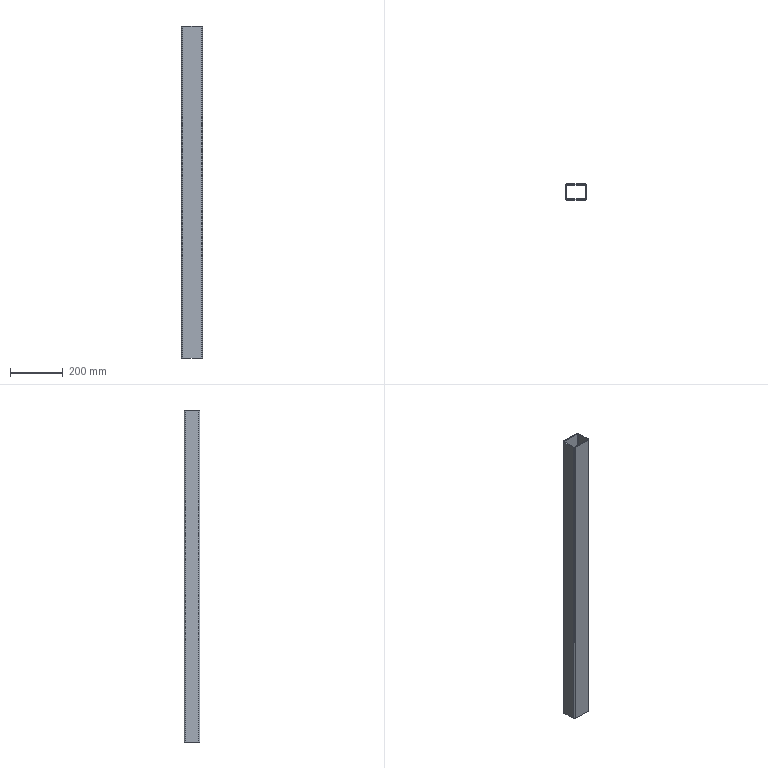Part | SolidWorks | features Extrusion 1, Fillet 1, Shell 1 | 1 solid | 18 faces | box 80 x 60 x 1264 mm | volume 993470 mm3 | plane 10 | cylinder 8 | commonest cylinder face diameters 4 x4 10 x4
STEP:
#1=CARTESIAN_POINT('',(40.,-25.,0.));
#2=VERTEX_POINT('',#1);
#3=CARTESIAN_POINT('',(40.,25.,0.));
#4=VERTEX_POINT('',#3);
#5=CARTESIAN_POINT('',(40.,30.,0.));
#6=DIRECTION('',(0.,1.,0.));
#7=VECTOR('',#6,1000.);
#8=LINE('',#5,#7);
#9=EDGE_CURVE('',#2,#4,#8,.T.);
#10=ORIENTED_EDGE('',*,*,#9,.F.);
#11=CARTESIAN_POINT('',(35.,-30.,0.));
#12=VERTEX_POINT('',#11);
#13=CARTESIAN_POINT('',(35.,-25.,0.));
#14=DIRECTION('',(0.,0.,-1.));
#15=DIRECTION('',(-1.,0.,0.));
#16=AXIS2_PLACEMENT_3D('',#13,#14,#15);
#17=CIRCLE('',#16,5.);
#18=EDGE_CURVE('',#2,#12,#17,.T.);
#19=ORIENTED_EDGE('',*,*,#18,.T.);
#20=CARTESIAN_POINT('',(-35.,-30.,0.));
#21=VERTEX_POINT('',#20);
#22=CARTESIAN_POINT('',(40.,-30.,0.));
#23=DIRECTION('',(1.,0.,0.));
#24=VECTOR('',#23,1000.);
#25=LINE('',#22,#24);
#26=EDGE_CURVE('',#21,#12,#25,.T.);
#27=ORIENTED_EDGE('',*,*,#26,.F.);
#28=CARTESIAN_POINT('',(-40.,-25.,0.));
#29=VERTEX_POINT('',#28);
#30=CARTESIAN_POINT('',(-35.,-25.,0.));
#31=DIRECTION('',(0.,0.,-1.));
#32=DIRECTION('',(-1.,0.,0.));
#33=AXIS2_PLACEMENT_3D('',#30,#31,#32);
#34=CIRCLE('',#33,5.);
#35=EDGE_CURVE('',#21,#29,#34,.T.);
#36=ORIENTED_EDGE('',*,*,#35,.T.);
#37=CARTESIAN_POINT('',(-40.,25.,0.));
#38=VERTEX_POINT('',#37);
#39=CARTESIAN_POINT('',(-40.,30.,0.));
#40=DIRECTION('',(0.,-1.,0.));
#41=VECTOR('',#40,1000.);
#42=LINE('',#39,#41);
#43=EDGE_CURVE('',#38,#29,#42,.T.);
#44=ORIENTED_EDGE('',*,*,#43,.F.);
#45=CARTESIAN_POINT('',(-35.,30.,0.));
#46=VERTEX_POINT('',#45);
#47=CARTESIAN_POINT('',(-35.,25.,0.));
#48=DIRECTION('',(0.,0.,-1.));
#49=DIRECTION('',(-1.,0.,0.));
#50=AXIS2_PLACEMENT_3D('',#47,#48,#49);
#51=CIRCLE('',#50,5.);
#52=EDGE_CURVE('',#38,#46,#51,.T.);
#53=ORIENTED_EDGE('',*,*,#52,.T.);
#54=CARTESIAN_POINT('',(35.,30.,0.));
#55=VERTEX_POINT('',#54);
#56=CARTESIAN_POINT('',(40.,30.,0.));
#57=DIRECTION('',(-1.,0.,0.));
#58=VECTOR('',#57,1000.);
#59=LINE('',#56,#58);
#60=EDGE_CURVE('',#55,#46,#59,.T.);
#61=ORIENTED_EDGE('',*,*,#60,.F.);
#62=CARTESIAN_POINT('',(35.,25.,0.));
#63=DIRECTION('',(0.,0.,-1.));
#64=DIRECTION('',(-1.,0.,0.));
#65=AXIS2_PLACEMENT_3D('',#62,#63,#64);
#66=CIRCLE('',#65,5.);
#67=EDGE_CURVE('',#55,#4,#66,.T.);
#68=ORIENTED_EDGE('',*,*,#67,.T.);
#69=EDGE_LOOP('',(#10,#19,#27,#36,#44,#53,#61,#68));
#70=FACE_OUTER_BOUND('',#69,.T.);
#71=CARTESIAN_POINT('',(37.,-25.,0.));
#72=VERTEX_POINT('',#71);
#73=CARTESIAN_POINT('',(35.,-27.,0.));
#74=VERTEX_POINT('',#73);
#75=CARTESIAN_POINT('',(35.,-25.,0.));
#76=DIRECTION('',(0.,0.,-1.));
#77=DIRECTION('',(-1.,0.,0.));
#78=AXIS2_PLACEMENT_3D('',#75,#76,#77);
#79=CIRCLE('',#78,2.);
#80=EDGE_CURVE('',#72,#74,#79,.T.);
#81=ORIENTED_EDGE('',*,*,#80,.F.);
#82=CARTESIAN_POINT('',(37.,25.,0.));
#83=VERTEX_POINT('',#82);
#84=CARTESIAN_POINT('',(37.,0.,0.));
#85=DIRECTION('',(0.,1.,0.));
#86=VECTOR('',#85,1000.);
#87=LINE('',#84,#86);
#88=EDGE_CURVE('',#72,#83,#87,.T.);
#89=ORIENTED_EDGE('',*,*,#88,.T.);
#90=CARTESIAN_POINT('',(35.,27.,0.));
#91=VERTEX_POINT('',#90);
#92=CARTESIAN_POINT('',(35.,25.,0.));
#93=DIRECTION('',(0.,0.,-1.));
#94=DIRECTION('',(-1.,0.,0.));
#95=AXIS2_PLACEMENT_3D('',#92,#93,#94);
#96=CIRCLE('',#95,2.);
#97=EDGE_CURVE('',#91,#83,#96,.T.);
#98=ORIENTED_EDGE('',*,*,#97,.F.);
#99=CARTESIAN_POINT('',(-35.,27.,0.));
#100=VERTEX_POINT('',#99);
#101=CARTESIAN_POINT('',(0.,27.,0.));
#102=DIRECTION('',(-1.,0.,0.));
#103=VECTOR('',#102,1000.);
#104=LINE('',#101,#103);
#105=EDGE_CURVE('',#91,#100,#104,.T.);
#106=ORIENTED_EDGE('',*,*,#105,.T.);
#107=CARTESIAN_POINT('',(-37.,25.,0.));
#108=VERTEX_POINT('',#107);
#109=CARTESIAN_POINT('',(-35.,25.,0.));
#110=DIRECTION('',(0.,0.,-1.));
#111=DIRECTION('',(-1.,0.,0.));
#112=AXIS2_PLACEMENT_3D('',#109,#110,#111);
#113=CIRCLE('',#112,2.);
#114=EDGE_CURVE('',#108,#100,#113,.T.);
#115=ORIENTED_EDGE('',*,*,#114,.F.);
#116=CARTESIAN_POINT('',(-37.,-25.,0.));
#117=VERTEX_POINT('',#116);
#118=CARTESIAN_POINT('',(-37.,0.,0.));
#119=DIRECTION('',(0.,-1.,0.));
#120=VECTOR('',#119,1000.);
#121=LINE('',#118,#120);
#122=EDGE_CURVE('',#108,#117,#121,.T.);
#123=ORIENTED_EDGE('',*,*,#122,.T.);
#124=CARTESIAN_POINT('',(-35.,-27.,0.));
#125=VERTEX_POINT('',#124);
#126=CARTESIAN_POINT('',(-35.,-25.,0.));
#127=DIRECTION('',(0.,0.,-1.));
#128=DIRECTION('',(-1.,0.,0.));
#129=AXIS2_PLACEMENT_3D('',#126,#127,#128);
#130=CIRCLE('',#129,2.);
#131=EDGE_CURVE('',#125,#117,#130,.T.);
#132=ORIENTED_EDGE('',*,*,#131,.F.);
#133=CARTESIAN_POINT('',(0.,-27.,0.));
#134=DIRECTION('',(1.,0.,0.));
#135=VECTOR('',#134,1000.);
#136=LINE('',#133,#135);
#137=EDGE_CURVE('',#125,#74,#136,.T.);
#138=ORIENTED_EDGE('',*,*,#137,.T.);
#139=EDGE_LOOP('',(#81,#89,#98,#106,#115,#123,#132,#138));
#140=FACE_BOUND('',#139,.T.);
#141=CARTESIAN_POINT('',(0.,0.,0.));
#142=DIRECTION('',(0.,0.,-1.));
#143=DIRECTION('',(-1.,0.,0.));
#144=AXIS2_PLACEMENT_3D('',#141,#142,#143);
#145=PLANE('',#144);
#146=ADVANCED_FACE('',(#70,#140),#145,.T.);
#147=ORIENTED_EDGE('',*,*,#43,.T.);
#148=CARTESIAN_POINT('',(-40.,-25.,1264.));
#149=VERTEX_POINT('',#148);
#150=CARTESIAN_POINT('',(-40.,-25.,1264.));
#151=DIRECTION('',(0.,0.,1.));
#152=VECTOR('',#151,1000.);
#153=LINE('',#150,#152);
#154=EDGE_CURVE('',#29,#149,#153,.T.);
#155=ORIENTED_EDGE('',*,*,#154,.T.);
#156=CARTESIAN_POINT('',(-40.,25.,1264.));
#157=VERTEX_POINT('',#156);
#158=CARTESIAN_POINT('',(-40.,30.,1264.));
#159=DIRECTION('',(0.,-1.,0.));
#160=VECTOR('',#159,1000.);
#161=LINE('',#158,#160);
#162=EDGE_CURVE('',#157,#149,#161,.T.);
#163=ORIENTED_EDGE('',*,*,#162,.F.);
#164=CARTESIAN_POINT('',(-40.,25.,1264.));
#165=DIRECTION('',(0.,0.,-1.));
#166=VECTOR('',#165,1000.);
#167=LINE('',#164,#166);
#168=EDGE_CURVE('',#157,#38,#167,.T.);
#169=ORIENTED_EDGE('',*,*,#168,.T.);
#170=EDGE_LOOP('',(#147,#155,#163,#169));
#171=FACE_OUTER_BOUND('',#170,.T.);
#172=CARTESIAN_POINT('',(-40.,30.,1264.));
#173=DIRECTION('',(1.,0.,0.));
#174=DIRECTION('',(0.,0.,-1.));
#175=AXIS2_PLACEMENT_3D('',#172,#173,#174);
#176=PLANE('',#175);
#177=ADVANCED_FACE('',(#171),#176,.F.);
#178=ORIENTED_EDGE('',*,*,#26,.T.);
#179=CARTESIAN_POINT('',(35.,-30.,1264.));
#180=VERTEX_POINT('',#179);
#181=CARTESIAN_POINT('',(35.,-30.,1264.));
#182=DIRECTION('',(0.,0.,1.));
#183=VECTOR('',#182,1000.);
#184=LINE('',#181,#183);
#185=EDGE_CURVE('',#12,#180,#184,.T.);
#186=ORIENTED_EDGE('',*,*,#185,.T.);
#187=CARTESIAN_POINT('',(-35.,-30.,1264.));
#188=VERTEX_POINT('',#187);
#189=CARTESIAN_POINT('',(40.,-30.,1264.));
#190=DIRECTION('',(1.,0.,0.));
#191=VECTOR('',#190,1000.);
#192=LINE('',#189,#191);
#193=EDGE_CURVE('',#188,#180,#192,.T.);
#194=ORIENTED_EDGE('',*,*,#193,.F.);
#195=CARTESIAN_POINT('',(-35.,-30.,1264.));
#196=DIRECTION('',(0.,0.,-1.));
#197=VECTOR('',#196,1000.);
#198=LINE('',#195,#197);
#199=EDGE_CURVE('',#188,#21,#198,.T.);
#200=ORIENTED_EDGE('',*,*,#199,.T.);
#201=EDGE_LOOP('',(#178,#186,#194,#200));
#202=FACE_OUTER_BOUND('',#201,.T.);
#203=CARTESIAN_POINT('',(40.,-30.,1264.));
#204=DIRECTION('',(0.,1.,0.));
#205=DIRECTION('',(-1.,0.,0.));
#206=AXIS2_PLACEMENT_3D('',#203,#204,#205);
#207=PLANE('',#206);
#208=ADVANCED_FACE('',(#202),#207,.F.);
#209=CARTESIAN_POINT('',(40.,-25.,1264.));
#210=VERTEX_POINT('',#209);
#211=CARTESIAN_POINT('',(40.,25.,1264.));
#212=VERTEX_POINT('',#211);
#213=CARTESIAN_POINT('',(40.,30.,1264.));
#214=DIRECTION('',(0.,1.,0.));
#215=VECTOR('',#214,1000.);
#216=LINE('',#213,#215);
#217=EDGE_CURVE('',#210,#212,#216,.T.);
#218=ORIENTED_EDGE('',*,*,#217,.F.);
#219=CARTESIAN_POINT('',(40.,-25.,1264.));
#220=DIRECTION('',(0.,0.,-1.));
#221=VECTOR('',#220,1000.);
#222=LINE('',#219,#221);
#223=EDGE_CURVE('',#210,#2,#222,.T.);
#224=ORIENTED_EDGE('',*,*,#223,.T.);
#225=ORIENTED_EDGE('',*,*,#9,.T.);
#226=CARTESIAN_POINT('',(40.,25.,1264.));
#227=DIRECTION('',(0.,0.,1.));
#228=VECTOR('',#227,1000.);
#229=LINE('',#226,#228);
#230=EDGE_CURVE('',#4,#212,#229,.T.);
#231=ORIENTED_EDGE('',*,*,#230,.T.);
#232=EDGE_LOOP('',(#218,#224,#225,#231));
#233=FACE_OUTER_BOUND('',#232,.T.);
#234=CARTESIAN_POINT('',(40.,30.,1264.));
#235=DIRECTION('',(-1.,0.,0.));
#236=DIRECTION('',(0.,-1.,0.));
#237=AXIS2_PLACEMENT_3D('',#234,#235,#236);
#238=PLANE('',#237);
#239=ADVANCED_FACE('',(#233),#238,.F.);
#240=ORIENTED_EDGE('',*,*,#60,.T.);
#241=CARTESIAN_POINT('',(-35.,30.,1264.));
#242=VERTEX_POINT('',#241);
#243=CARTESIAN_POINT('',(-35.,30.,1264.));
#244=DIRECTION('',(0.,0.,1.));
#245=VECTOR('',#244,1000.);
#246=LINE('',#243,#245);
#247=EDGE_CURVE('',#46,#242,#246,.T.);
#248=ORIENTED_EDGE('',*,*,#247,.T.);
#249=CARTESIAN_POINT('',(35.,30.,1264.));
#250=VERTEX_POINT('',#249);
#251=CARTESIAN_POINT('',(40.,30.,1264.));
#252=DIRECTION('',(-1.,0.,0.));
#253=VECTOR('',#252,1000.);
#254=LINE('',#251,#253);
#255=EDGE_CURVE('',#250,#242,#254,.T.);
#256=ORIENTED_EDGE('',*,*,#255,.F.);
#257=CARTESIAN_POINT('',(35.,30.,1264.));
#258=DIRECTION('',(0.,0.,-1.));
#259=VECTOR('',#258,1000.);
#260=LINE('',#257,#259);
#261=EDGE_CURVE('',#250,#55,#260,.T.);
#262=ORIENTED_EDGE('',*,*,#261,.T.);
#263=EDGE_LOOP('',(#240,#248,#256,#262));
#264=FACE_OUTER_BOUND('',#263,.T.);
#265=CARTESIAN_POINT('',(40.,30.,1264.));
#266=DIRECTION('',(0.,-1.,0.));
#267=DIRECTION('',(1.,0.,0.));
#268=AXIS2_PLACEMENT_3D('',#265,#266,#267);
#269=PLANE('',#268);
#270=ADVANCED_FACE('',(#264),#269,.F.);
#271=CARTESIAN_POINT('',(-35.,-27.,1264.));
#272=VERTEX_POINT('',#271);
#273=CARTESIAN_POINT('',(35.,-27.,1264.));
#274=VERTEX_POINT('',#273);
#275=CARTESIAN_POINT('',(0.,-27.,1264.));
#276=DIRECTION('',(1.,0.,0.));
#277=VECTOR('',#276,1000.);
#278=LINE('',#275,#277);
#279=EDGE_CURVE('',#272,#274,#278,.T.);
#280=ORIENTED_EDGE('',*,*,#279,.F.);
#281=CARTESIAN_POINT('',(-37.,-25.,1264.));
#282=VERTEX_POINT('',#281);
#283=CARTESIAN_POINT('',(-35.,-25.,1264.));
#284=DIRECTION('',(0.,0.,1.));
#285=DIRECTION('',(-1.,0.,0.));
#286=AXIS2_PLACEMENT_3D('',#283,#284,#285);
#287=CIRCLE('',#286,2.);
#288=EDGE_CURVE('',#282,#272,#287,.T.);
#289=ORIENTED_EDGE('',*,*,#288,.F.);
#290=CARTESIAN_POINT('',(-37.,25.,1264.));
#291=VERTEX_POINT('',#290);
#292=CARTESIAN_POINT('',(-37.,0.,1264.));
#293=DIRECTION('',(0.,-1.,0.));
#294=VECTOR('',#293,1000.);
#295=LINE('',#292,#294);
#296=EDGE_CURVE('',#291,#282,#295,.T.);
#297=ORIENTED_EDGE('',*,*,#296,.F.);
#298=CARTESIAN_POINT('',(-35.,27.,1264.));
#299=VERTEX_POINT('',#298);
#300=CARTESIAN_POINT('',(-35.,25.,1264.));
#301=DIRECTION('',(0.,0.,1.));
#302=DIRECTION('',(-1.,0.,0.));
#303=AXIS2_PLACEMENT_3D('',#300,#301,#302);
#304=CIRCLE('',#303,2.);
#305=EDGE_CURVE('',#299,#291,#304,.T.);
#306=ORIENTED_EDGE('',*,*,#305,.F.);
#307=CARTESIAN_POINT('',(35.,27.,1264.));
#308=VERTEX_POINT('',#307);
#309=CARTESIAN_POINT('',(0.,27.,1264.));
#310=DIRECTION('',(-1.,0.,0.));
#311=VECTOR('',#310,1000.);
#312=LINE('',#309,#311);
#313=EDGE_CURVE('',#308,#299,#312,.T.);
#314=ORIENTED_EDGE('',*,*,#313,.F.);
#315=CARTESIAN_POINT('',(37.,25.,1264.));
#316=VERTEX_POINT('',#315);
#317=CARTESIAN_POINT('',(35.,25.,1264.));
#318=DIRECTION('',(0.,0.,1.));
#319=DIRECTION('',(-1.,0.,0.));
#320=AXIS2_PLACEMENT_3D('',#317,#318,#319);
#321=CIRCLE('',#320,2.);
#322=EDGE_CURVE('',#316,#308,#321,.T.);
#323=ORIENTED_EDGE('',*,*,#322,.F.);
#324=CARTESIAN_POINT('',(37.,-25.,1264.));
#325=VERTEX_POINT('',#324);
#326=CARTESIAN_POINT('',(37.,0.,1264.));
#327=DIRECTION('',(0.,1.,0.));
#328=VECTOR('',#327,1000.);
#329=LINE('',#326,#328);
#330=EDGE_CURVE('',#325,#316,#329,.T.);
#331=ORIENTED_EDGE('',*,*,#330,.F.);
#332=CARTESIAN_POINT('',(35.,-25.,1264.));
#333=DIRECTION('',(0.,0.,1.));
#334=DIRECTION('',(-1.,0.,0.));
#335=AXIS2_PLACEMENT_3D('',#332,#333,#334);
#336=CIRCLE('',#335,2.);
#337=EDGE_CURVE('',#274,#325,#336,.T.);
#338=ORIENTED_EDGE('',*,*,#337,.F.);
#339=EDGE_LOOP('',(#280,#289,#297,#306,#314,#323,#331,#338));
#340=FACE_BOUND('',#339,.T.);
#341=ORIENTED_EDGE('',*,*,#193,.T.);
#342=CARTESIAN_POINT('',(35.,-25.,1264.));
#343=DIRECTION('',(0.,0.,1.));
#344=DIRECTION('',(-1.,0.,0.));
#345=AXIS2_PLACEMENT_3D('',#342,#343,#344);
#346=CIRCLE('',#345,5.);
#347=EDGE_CURVE('',#180,#210,#346,.T.);
#348=ORIENTED_EDGE('',*,*,#347,.T.);
#349=ORIENTED_EDGE('',*,*,#217,.T.);
#350=CARTESIAN_POINT('',(35.,25.,1264.));
#351=DIRECTION('',(0.,0.,1.));
#352=DIRECTION('',(-1.,0.,0.));
#353=AXIS2_PLACEMENT_3D('',#350,#351,#352);
#354=CIRCLE('',#353,5.);
#355=EDGE_CURVE('',#212,#250,#354,.T.);
#356=ORIENTED_EDGE('',*,*,#355,.T.);
#357=ORIENTED_EDGE('',*,*,#255,.T.);
#358=CARTESIAN_POINT('',(-35.,25.,1264.));
#359=DIRECTION('',(0.,0.,1.));
#360=DIRECTION('',(-1.,0.,0.));
#361=AXIS2_PLACEMENT_3D('',#358,#359,#360);
#362=CIRCLE('',#361,5.);
#363=EDGE_CURVE('',#242,#157,#362,.T.);
#364=ORIENTED_EDGE('',*,*,#363,.T.);
#365=ORIENTED_EDGE('',*,*,#162,.T.);
#366=CARTESIAN_POINT('',(-35.,-25.,1264.));
#367=DIRECTION('',(0.,0.,1.));
#368=DIRECTION('',(-1.,0.,0.));
#369=AXIS2_PLACEMENT_3D('',#366,#367,#368);
#370=CIRCLE('',#369,5.);
#371=EDGE_CURVE('',#149,#188,#370,.T.);
#372=ORIENTED_EDGE('',*,*,#371,.T.);
#373=EDGE_LOOP('',(#341,#348,#349,#356,#357,#364,#365,#372));
#374=FACE_OUTER_BOUND('',#373,.T.);
#375=CARTESIAN_POINT('',(0.,0.,1264.));
#376=DIRECTION('',(0.,0.,-1.));
#377=DIRECTION('',(-1.,0.,0.));
#378=AXIS2_PLACEMENT_3D('',#375,#376,#377);
#379=PLANE('',#378);
#380=ADVANCED_FACE('',(#340,#374),#379,.F.);
#381=ORIENTED_EDGE('',*,*,#347,.F.);
#382=ORIENTED_EDGE('',*,*,#185,.F.);
#383=ORIENTED_EDGE('',*,*,#18,.F.);
#384=ORIENTED_EDGE('',*,*,#223,.F.);
#385=EDGE_LOOP('',(#381,#382,#383,#384));
#386=FACE_OUTER_BOUND('',#385,.T.);
#387=CARTESIAN_POINT('',(35.,-25.,1264.));
#388=DIRECTION('',(0.,0.,-1.));
#389=DIRECTION('',(-1.,0.,0.));
#390=AXIS2_PLACEMENT_3D('',#387,#388,#389);
#391=CYLINDRICAL_SURFACE('',#390,5.);
#392=ADVANCED_FACE('',(#386),#391,.T.);
#393=ORIENTED_EDGE('',*,*,#371,.F.);
#394=ORIENTED_EDGE('',*,*,#154,.F.);
#395=ORIENTED_EDGE('',*,*,#35,.F.);
#396=ORIENTED_EDGE('',*,*,#199,.F.);
#397=EDGE_LOOP('',(#393,#394,#395,#396));
#398=FACE_OUTER_BOUND('',#397,.T.);
#399=CARTESIAN_POINT('',(-35.,-25.,1264.));
#400=DIRECTION('',(0.,0.,-1.));
#401=DIRECTION('',(-1.,0.,0.));
#402=AXIS2_PLACEMENT_3D('',#399,#400,#401);
#403=CYLINDRICAL_SURFACE('',#402,5.);
#404=ADVANCED_FACE('',(#398),#403,.T.);
#405=ORIENTED_EDGE('',*,*,#363,.F.);
#406=ORIENTED_EDGE('',*,*,#247,.F.);
#407=ORIENTED_EDGE('',*,*,#52,.F.);
#408=ORIENTED_EDGE('',*,*,#168,.F.);
#409=EDGE_LOOP('',(#405,#406,#407,#408));
#410=FACE_OUTER_BOUND('',#409,.T.);
#411=CARTESIAN_POINT('',(-35.,25.,1264.));
#412=DIRECTION('',(0.,0.,-1.));
#413=DIRECTION('',(-1.,0.,0.));
#414=AXIS2_PLACEMENT_3D('',#411,#412,#413);
#415=CYLINDRICAL_SURFACE('',#414,5.);
#416=ADVANCED_FACE('',(#410),#415,.T.);
#417=ORIENTED_EDGE('',*,*,#355,.F.);
#418=ORIENTED_EDGE('',*,*,#230,.F.);
#419=ORIENTED_EDGE('',*,*,#67,.F.);
#420=ORIENTED_EDGE('',*,*,#261,.F.);
#421=EDGE_LOOP('',(#417,#418,#419,#420));
#422=FACE_OUTER_BOUND('',#421,.T.);
#423=CARTESIAN_POINT('',(35.,25.,1264.));
#424=DIRECTION('',(0.,0.,-1.));
#425=DIRECTION('',(-1.,0.,0.));
#426=AXIS2_PLACEMENT_3D('',#423,#424,#425);
#427=CYLINDRICAL_SURFACE('',#426,5.);
#428=ADVANCED_FACE('',(#422),#427,.T.);
#429=ORIENTED_EDGE('',*,*,#122,.F.);
#430=CARTESIAN_POINT('',(-37.,25.,1264.));
#431=DIRECTION('',(0.,0.,-1.));
#432=VECTOR('',#431,1000.);
#433=LINE('',#430,#432);
#434=EDGE_CURVE('',#291,#108,#433,.T.);
#435=ORIENTED_EDGE('',*,*,#434,.F.);
#436=ORIENTED_EDGE('',*,*,#296,.T.);
#437=CARTESIAN_POINT('',(-37.,-25.,1264.));
#438=DIRECTION('',(0.,0.,1.));
#439=VECTOR('',#438,1000.);
#440=LINE('',#437,#439);
#441=EDGE_CURVE('',#117,#282,#440,.T.);
#442=ORIENTED_EDGE('',*,*,#441,.F.);
#443=EDGE_LOOP('',(#429,#435,#436,#442));
#444=FACE_OUTER_BOUND('',#443,.T.);
#445=CARTESIAN_POINT('',(-37.,30.,1264.));
#446=DIRECTION('',(1.,0.,0.));
#447=DIRECTION('',(0.,0.,-1.));
#448=AXIS2_PLACEMENT_3D('',#445,#446,#447);
#449=PLANE('',#448);
#450=ADVANCED_FACE('',(#444),#449,.T.);
#451=ORIENTED_EDGE('',*,*,#137,.F.);
#452=CARTESIAN_POINT('',(-35.,-27.,1264.));
#453=DIRECTION('',(0.,0.,-1.));
#454=VECTOR('',#453,1000.);
#455=LINE('',#452,#454);
#456=EDGE_CURVE('',#272,#125,#455,.T.);
#457=ORIENTED_EDGE('',*,*,#456,.F.);
#458=ORIENTED_EDGE('',*,*,#279,.T.);
#459=CARTESIAN_POINT('',(35.,-27.,1264.));
#460=DIRECTION('',(0.,0.,1.));
#461=VECTOR('',#460,1000.);
#462=LINE('',#459,#461);
#463=EDGE_CURVE('',#74,#274,#462,.T.);
#464=ORIENTED_EDGE('',*,*,#463,.F.);
#465=EDGE_LOOP('',(#451,#457,#458,#464));
#466=FACE_OUTER_BOUND('',#465,.T.);
#467=CARTESIAN_POINT('',(40.,-27.,1264.));
#468=DIRECTION('',(0.,1.,0.));
#469=DIRECTION('',(-1.,0.,0.));
#470=AXIS2_PLACEMENT_3D('',#467,#468,#469);
#471=PLANE('',#470);
#472=ADVANCED_FACE('',(#466),#471,.T.);
#473=ORIENTED_EDGE('',*,*,#330,.T.);
#474=CARTESIAN_POINT('',(37.,25.,1264.));
#475=DIRECTION('',(0.,0.,1.));
#476=VECTOR('',#475,1000.);
#477=LINE('',#474,#476);
#478=EDGE_CURVE('',#83,#316,#477,.T.);
#479=ORIENTED_EDGE('',*,*,#478,.F.);
#480=ORIENTED_EDGE('',*,*,#88,.F.);
#481=CARTESIAN_POINT('',(37.,-25.,1264.));
#482=DIRECTION('',(0.,0.,-1.));
#483=VECTOR('',#482,1000.);
#484=LINE('',#481,#483);
#485=EDGE_CURVE('',#325,#72,#484,.T.);
#486=ORIENTED_EDGE('',*,*,#485,.F.);
#487=EDGE_LOOP('',(#473,#479,#480,#486));
#488=FACE_OUTER_BOUND('',#487,.T.);
#489=CARTESIAN_POINT('',(37.,30.,1264.));
#490=DIRECTION('',(-1.,0.,0.));
#491=DIRECTION('',(0.,-1.,0.));
#492=AXIS2_PLACEMENT_3D('',#489,#490,#491);
#493=PLANE('',#492);
#494=ADVANCED_FACE('',(#488),#493,.T.);
#495=ORIENTED_EDGE('',*,*,#105,.F.);
#496=CARTESIAN_POINT('',(35.,27.,1264.));
#497=DIRECTION('',(0.,0.,-1.));
#498=VECTOR('',#497,1000.);
#499=LINE('',#496,#498);
#500=EDGE_CURVE('',#308,#91,#499,.T.);
#501=ORIENTED_EDGE('',*,*,#500,.F.);
#502=ORIENTED_EDGE('',*,*,#313,.T.);
#503=CARTESIAN_POINT('',(-35.,27.,1264.));
#504=DIRECTION('',(0.,0.,1.));
#505=VECTOR('',#504,1000.);
#506=LINE('',#503,#505);
#507=EDGE_CURVE('',#100,#299,#506,.T.);
#508=ORIENTED_EDGE('',*,*,#507,.F.);
#509=EDGE_LOOP('',(#495,#501,#502,#508));
#510=FACE_OUTER_BOUND('',#509,.T.);
#511=CARTESIAN_POINT('',(40.,27.,1264.));
#512=DIRECTION('',(0.,-1.,0.));
#513=DIRECTION('',(1.,0.,0.));
#514=AXIS2_PLACEMENT_3D('',#511,#512,#513);
#515=PLANE('',#514);
#516=ADVANCED_FACE('',(#510),#515,.T.);
#517=ORIENTED_EDGE('',*,*,#337,.T.);
#518=ORIENTED_EDGE('',*,*,#485,.T.);
#519=ORIENTED_EDGE('',*,*,#80,.T.);
#520=ORIENTED_EDGE('',*,*,#463,.T.);
#521=EDGE_LOOP('',(#517,#518,#519,#520));
#522=FACE_OUTER_BOUND('',#521,.T.);
#523=CARTESIAN_POINT('',(35.,-25.,1264.));
#524=DIRECTION('',(0.,0.,-1.));
#525=DIRECTION('',(-1.,0.,0.));
#526=AXIS2_PLACEMENT_3D('',#523,#524,#525);
#527=CYLINDRICAL_SURFACE('',#526,2.);
#528=ADVANCED_FACE('',(#522),#527,.F.);
#529=ORIENTED_EDGE('',*,*,#288,.T.);
#530=ORIENTED_EDGE('',*,*,#456,.T.);
#531=ORIENTED_EDGE('',*,*,#131,.T.);
#532=ORIENTED_EDGE('',*,*,#441,.T.);
#533=EDGE_LOOP('',(#529,#530,#531,#532));
#534=FACE_OUTER_BOUND('',#533,.T.);
#535=CARTESIAN_POINT('',(-35.,-25.,1264.));
#536=DIRECTION('',(0.,0.,-1.));
#537=DIRECTION('',(-1.,0.,0.));
#538=AXIS2_PLACEMENT_3D('',#535,#536,#537);
#539=CYLINDRICAL_SURFACE('',#538,2.);
#540=ADVANCED_FACE('',(#534),#539,.F.);
#541=ORIENTED_EDGE('',*,*,#305,.T.);
#542=ORIENTED_EDGE('',*,*,#434,.T.);
#543=ORIENTED_EDGE('',*,*,#114,.T.);
#544=ORIENTED_EDGE('',*,*,#507,.T.);
#545=EDGE_LOOP('',(#541,#542,#543,#544));
#546=FACE_OUTER_BOUND('',#545,.T.);
#547=CARTESIAN_POINT('',(-35.,25.,1264.));
#548=DIRECTION('',(0.,0.,-1.));
#549=DIRECTION('',(-1.,0.,0.));
#550=AXIS2_PLACEMENT_3D('',#547,#548,#549);
#551=CYLINDRICAL_SURFACE('',#550,2.);
#552=ADVANCED_FACE('',(#546),#551,.F.);
#553=ORIENTED_EDGE('',*,*,#322,.T.);
#554=ORIENTED_EDGE('',*,*,#500,.T.);
#555=ORIENTED_EDGE('',*,*,#97,.T.);
#556=ORIENTED_EDGE('',*,*,#478,.T.);
#557=EDGE_LOOP('',(#553,#554,#555,#556));
#558=FACE_OUTER_BOUND('',#557,.T.);
#559=CARTESIAN_POINT('',(35.,25.,1264.));
#560=DIRECTION('',(0.,0.,-1.));
#561=DIRECTION('',(-1.,0.,0.));
#562=AXIS2_PLACEMENT_3D('',#559,#560,#561);
#563=CYLINDRICAL_SURFACE('',#562,2.);
#564=ADVANCED_FACE('',(#558),#563,.F.);
#565=CLOSED_SHELL('',(#146,#177,#208,#239,#270,#380,#392,#404,#416,#428,#450,#472,#494,#516,#528,#540,#552,#564));
#566=MANIFOLD_SOLID_BREP('',#565);
#567=CARTESIAN_POINT('',(0.,0.,0.));
#568=DIRECTION('',(0.,0.,1.));
#569=DIRECTION('',(1.,0.,0.));
#570=AXIS2_PLACEMENT_3D('',#567,#568,#569);
#571=(LENGTH_UNIT()NAMED_UNIT(*)SI_UNIT(.MILLI.,.METRE.));
#572=UNCERTAINTY_MEASURE_WITH_UNIT(LENGTH_MEASURE(0.00001),#571,'','');
#573=(NAMED_UNIT(*)PLANE_ANGLE_UNIT()SI_UNIT($,.RADIAN.));
#574=(NAMED_UNIT(*)SI_UNIT($,.STERADIAN.)SOLID_ANGLE_UNIT());
#575=(GEOMETRIC_REPRESENTATION_CONTEXT(3)GLOBAL_UNCERTAINTY_ASSIGNED_CONTEXT((#572))GLOBAL_UNIT_ASSIGNED_CONTEXT((#571,#573,#574))REPRESENTATION_CONTEXT('',''));
#576=ADVANCED_BREP_SHAPE_REPRESENTATION('',(#566,#570),#575);